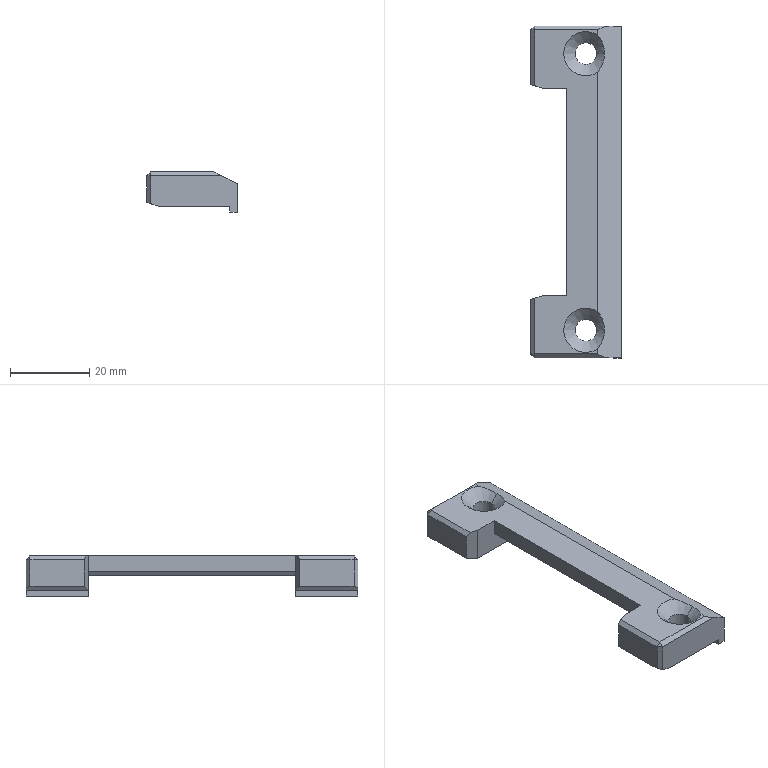Part | NX | features BREP 1 | 1 solid | 38 faces | box 23 x 84 x 10.2 mm | volume 8537 mm3 | plane 30 | cone 4 | cylinder 4 | commonest cylinder face diameters 5.5 x4
STEP:
#1=CARTESIAN_POINT('',(108.084,-207.077,2.15));
#2=VERTEX_POINT('',#1);
#3=CARTESIAN_POINT('',(113.584,-207.077,2.15));
#4=VERTEX_POINT('',#3);
#5=CARTESIAN_POINT('',(110.834,-207.077,2.15));
#6=DIRECTION('',(0.,0.,1.));
#7=DIRECTION('',(1.,0.,0.));
#8=AXIS2_PLACEMENT_3D('',#5,#6,#7);
#9=CIRCLE('',#8,2.75);
#10=EDGE_CURVE('',#2,#4,#9,.T.);
#11=ORIENTED_EDGE('',*,*,#10,.F.);
#12=CARTESIAN_POINT('',(105.234,-207.077,5.));
#13=VERTEX_POINT('',#12);
#14=CARTESIAN_POINT('',(105.234,-207.077,5.));
#15=DIRECTION('',(-0.7071,0.,0.7071));
#16=VECTOR('',#15,1000.);
#17=LINE('',#14,#16);
#18=EDGE_CURVE('',#13,#2,#17,.F.);
#19=ORIENTED_EDGE('',*,*,#18,.F.);
#20=CARTESIAN_POINT('',(113.834,-211.806,5.));
#21=VERTEX_POINT('',#20);
#22=CARTESIAN_POINT('',(110.834,-207.077,5.));
#23=DIRECTION('',(0.,0.,1.));
#24=DIRECTION('',(1.,0.,0.));
#25=AXIS2_PLACEMENT_3D('',#22,#23,#24);
#26=CIRCLE('',#25,5.6);
#27=EDGE_CURVE('',#13,#21,#26,.T.);
#28=ORIENTED_EDGE('',*,*,#27,.T.);
#29=CARTESIAN_POINT('',(115.568,-207.077,4.133));
#30=VERTEX_POINT('',#29);
#31=CARTESIAN_POINT('',(113.834,-211.806,5.));
#32=CARTESIAN_POINT('',(114.971,-210.411,4.432));
#33=CARTESIAN_POINT('',(115.568,-208.784,4.133));
#34=CARTESIAN_POINT('',(115.568,-207.077,4.133));
#35=(BOUNDED_CURVE()B_SPLINE_CURVE(3,(#31,#32,#33,#34),.UNSPECIFIED.,.F.,.F.)B_SPLINE_CURVE_WITH_KNOTS((4,4),(2.527,3.142),.UNSPECIFIED.)CURVE()GEOMETRIC_REPRESENTATION_ITEM()RATIONAL_B_SPLINE_CURVE((1.,0.9688,0.9688,1.))REPRESENTATION_ITEM(''));
#36=EDGE_CURVE('',#21,#30,#35,.T.);
#37=ORIENTED_EDGE('',*,*,#36,.T.);
#38=CARTESIAN_POINT('',(116.434,-207.077,5.));
#39=DIRECTION('',(0.7071,0.,0.7071));
#40=VECTOR('',#39,1000.);
#41=LINE('',#38,#40);
#42=EDGE_CURVE('',#30,#4,#41,.F.);
#43=ORIENTED_EDGE('',*,*,#42,.T.);
#44=EDGE_LOOP('',(#11,#19,#28,#37,#43));
#45=FACE_BOUND('',#44,.T.);
#46=CARTESIAN_POINT('',(110.834,-207.077,5.));
#47=DIRECTION('',(0.,0.,1.));
#48=DIRECTION('',(1.,0.,0.));
#49=AXIS2_PLACEMENT_3D('',#46,#47,#48);
#50=CONICAL_SURFACE('',#49,5.6,0.7854);
#51=ADVANCED_FACE('',(#45),#50,.F.);
#52=CARTESIAN_POINT('',(113.584,-207.077,-3.7));
#53=VERTEX_POINT('',#52);
#54=CARTESIAN_POINT('',(108.084,-207.077,-3.7));
#55=VERTEX_POINT('',#54);
#56=CARTESIAN_POINT('',(110.834,-207.077,-3.7));
#57=DIRECTION('',(0.,0.,-1.));
#58=DIRECTION('',(-1.,0.,0.));
#59=AXIS2_PLACEMENT_3D('',#56,#57,#58);
#60=CIRCLE('',#59,2.75);
#61=EDGE_CURVE('',#53,#55,#60,.T.);
#62=ORIENTED_EDGE('',*,*,#61,.T.);
#63=CARTESIAN_POINT('',(108.084,-207.077,5.));
#64=DIRECTION('',(0.,0.,1.));
#65=VECTOR('',#64,1000.);
#66=LINE('',#63,#65);
#67=EDGE_CURVE('',#2,#55,#66,.F.);
#68=ORIENTED_EDGE('',*,*,#67,.F.);
#69=ORIENTED_EDGE('',*,*,#10,.T.);
#70=CARTESIAN_POINT('',(113.584,-207.077,5.));
#71=DIRECTION('',(0.,0.,1.));
#72=VECTOR('',#71,1000.);
#73=LINE('',#70,#72);
#74=EDGE_CURVE('',#4,#53,#73,.F.);
#75=ORIENTED_EDGE('',*,*,#74,.T.);
#76=EDGE_LOOP('',(#62,#68,#69,#75));
#77=FACE_BOUND('',#76,.T.);
#78=CARTESIAN_POINT('',(110.834,-207.077,5.));
#79=DIRECTION('',(0.,0.,1.));
#80=DIRECTION('',(1.,0.,0.));
#81=AXIS2_PLACEMENT_3D('',#78,#79,#80);
#82=CYLINDRICAL_SURFACE('',#81,2.75);
#83=ADVANCED_FACE('',(#77),#82,.F.);
#84=CARTESIAN_POINT('',(108.084,-277.077,2.15));
#85=VERTEX_POINT('',#84);
#86=CARTESIAN_POINT('',(113.584,-277.077,2.15));
#87=VERTEX_POINT('',#86);
#88=CARTESIAN_POINT('',(110.834,-277.077,2.15));
#89=DIRECTION('',(0.,0.,1.));
#90=DIRECTION('',(1.,0.,0.));
#91=AXIS2_PLACEMENT_3D('',#88,#89,#90);
#92=CIRCLE('',#91,2.75);
#93=EDGE_CURVE('',#85,#87,#92,.T.);
#94=ORIENTED_EDGE('',*,*,#93,.F.);
#95=CARTESIAN_POINT('',(105.234,-277.077,5.));
#96=VERTEX_POINT('',#95);
#97=CARTESIAN_POINT('',(105.234,-277.077,5.));
#98=DIRECTION('',(-0.7071,0.,0.7071));
#99=VECTOR('',#98,1000.);
#100=LINE('',#97,#99);
#101=EDGE_CURVE('',#96,#85,#100,.F.);
#102=ORIENTED_EDGE('',*,*,#101,.F.);
#103=CARTESIAN_POINT('',(113.834,-281.806,5.));
#104=VERTEX_POINT('',#103);
#105=CARTESIAN_POINT('',(110.834,-277.077,5.));
#106=DIRECTION('',(0.,0.,1.));
#107=DIRECTION('',(1.,0.,0.));
#108=AXIS2_PLACEMENT_3D('',#105,#106,#107);
#109=CIRCLE('',#108,5.6);
#110=EDGE_CURVE('',#96,#104,#109,.T.);
#111=ORIENTED_EDGE('',*,*,#110,.T.);
#112=CARTESIAN_POINT('',(115.568,-277.077,4.133));
#113=VERTEX_POINT('',#112);
#114=CARTESIAN_POINT('',(113.834,-281.806,5.));
#115=CARTESIAN_POINT('',(114.971,-280.411,4.432));
#116=CARTESIAN_POINT('',(115.568,-278.784,4.133));
#117=CARTESIAN_POINT('',(115.568,-277.077,4.133));
#118=(BOUNDED_CURVE()B_SPLINE_CURVE(3,(#114,#115,#116,#117),.UNSPECIFIED.,.F.,.F.)B_SPLINE_CURVE_WITH_KNOTS((4,4),(2.527,3.142),.UNSPECIFIED.)CURVE()GEOMETRIC_REPRESENTATION_ITEM()RATIONAL_B_SPLINE_CURVE((1.,0.9688,0.9688,1.))REPRESENTATION_ITEM(''));
#119=EDGE_CURVE('',#104,#113,#118,.T.);
#120=ORIENTED_EDGE('',*,*,#119,.T.);
#121=CARTESIAN_POINT('',(116.434,-277.077,5.));
#122=DIRECTION('',(0.7071,0.,0.7071));
#123=VECTOR('',#122,1000.);
#124=LINE('',#121,#123);
#125=EDGE_CURVE('',#113,#87,#124,.F.);
#126=ORIENTED_EDGE('',*,*,#125,.T.);
#127=EDGE_LOOP('',(#94,#102,#111,#120,#126));
#128=FACE_BOUND('',#127,.T.);
#129=CARTESIAN_POINT('',(110.834,-277.077,5.));
#130=DIRECTION('',(0.,0.,1.));
#131=DIRECTION('',(1.,0.,0.));
#132=AXIS2_PLACEMENT_3D('',#129,#130,#131);
#133=CONICAL_SURFACE('',#132,5.6,0.7854);
#134=ADVANCED_FACE('',(#128),#133,.F.);
#135=CARTESIAN_POINT('',(108.084,-277.077,-3.7));
#136=VERTEX_POINT('',#135);
#137=CARTESIAN_POINT('',(113.584,-277.077,-3.7));
#138=VERTEX_POINT('',#137);
#139=CARTESIAN_POINT('',(110.834,-277.077,-3.7));
#140=DIRECTION('',(0.,0.,1.));
#141=DIRECTION('',(1.,0.,0.));
#142=AXIS2_PLACEMENT_3D('',#139,#140,#141);
#143=CIRCLE('',#142,2.75);
#144=EDGE_CURVE('',#136,#138,#143,.T.);
#145=ORIENTED_EDGE('',*,*,#144,.F.);
#146=CARTESIAN_POINT('',(108.084,-277.077,5.));
#147=DIRECTION('',(0.,0.,1.));
#148=VECTOR('',#147,1000.);
#149=LINE('',#146,#148);
#150=EDGE_CURVE('',#85,#136,#149,.F.);
#151=ORIENTED_EDGE('',*,*,#150,.F.);
#152=ORIENTED_EDGE('',*,*,#93,.T.);
#153=CARTESIAN_POINT('',(113.584,-277.077,5.));
#154=DIRECTION('',(0.,0.,1.));
#155=VECTOR('',#154,1000.);
#156=LINE('',#153,#155);
#157=EDGE_CURVE('',#87,#138,#156,.F.);
#158=ORIENTED_EDGE('',*,*,#157,.T.);
#159=EDGE_LOOP('',(#145,#151,#152,#158));
#160=FACE_BOUND('',#159,.T.);
#161=CARTESIAN_POINT('',(110.834,-277.077,5.));
#162=DIRECTION('',(0.,0.,1.));
#163=DIRECTION('',(1.,0.,0.));
#164=AXIS2_PLACEMENT_3D('',#161,#162,#163);
#165=CYLINDRICAL_SURFACE('',#164,2.75);
#166=ADVANCED_FACE('',(#160),#165,.F.);
#167=CARTESIAN_POINT('',(97.834,-268.994,5.));
#168=VERTEX_POINT('',#167);
#169=CARTESIAN_POINT('',(97.834,-283.077,5.));
#170=VERTEX_POINT('',#169);
#171=CARTESIAN_POINT('',(97.834,-284.077,5.));
#172=DIRECTION('',(0.,-1.,0.));
#173=VECTOR('',#172,1000.);
#174=LINE('',#171,#173);
#175=EDGE_CURVE('',#168,#170,#174,.T.);
#176=ORIENTED_EDGE('',*,*,#175,.T.);
#177=CARTESIAN_POINT('',(113.834,-283.077,5.));
#178=VERTEX_POINT('',#177);
#179=CARTESIAN_POINT('',(105.834,-283.077,5.));
#180=DIRECTION('',(1.,0.,0.));
#181=VECTOR('',#180,1000.);
#182=LINE('',#179,#181);
#183=EDGE_CURVE('',#170,#178,#182,.T.);
#184=ORIENTED_EDGE('',*,*,#183,.T.);
#185=CARTESIAN_POINT('',(113.834,-200.077,5.));
#186=DIRECTION('',(0.,1.,0.));
#187=VECTOR('',#186,1000.);
#188=LINE('',#185,#187);
#189=EDGE_CURVE('',#178,#104,#188,.T.);
#190=ORIENTED_EDGE('',*,*,#189,.T.);
#191=ORIENTED_EDGE('',*,*,#110,.F.);
#192=CARTESIAN_POINT('',(113.834,-272.349,5.));
#193=VERTEX_POINT('',#192);
#194=CARTESIAN_POINT('',(110.834,-277.077,5.));
#195=DIRECTION('',(0.,0.,1.));
#196=DIRECTION('',(1.,0.,0.));
#197=AXIS2_PLACEMENT_3D('',#194,#195,#196);
#198=CIRCLE('',#197,5.6);
#199=EDGE_CURVE('',#193,#96,#198,.T.);
#200=ORIENTED_EDGE('',*,*,#199,.F.);
#201=CARTESIAN_POINT('',(113.834,-200.077,5.));
#202=DIRECTION('',(0.,1.,0.));
#203=VECTOR('',#202,1000.);
#204=LINE('',#201,#203);
#205=EDGE_CURVE('',#193,#21,#204,.T.);
#206=ORIENTED_EDGE('',*,*,#205,.T.);
#207=ORIENTED_EDGE('',*,*,#27,.F.);
#208=CARTESIAN_POINT('',(113.834,-202.349,5.));
#209=VERTEX_POINT('',#208);
#210=CARTESIAN_POINT('',(110.834,-207.077,5.));
#211=DIRECTION('',(0.,0.,1.));
#212=DIRECTION('',(1.,0.,0.));
#213=AXIS2_PLACEMENT_3D('',#210,#211,#212);
#214=CIRCLE('',#213,5.6);
#215=EDGE_CURVE('',#209,#13,#214,.T.);
#216=ORIENTED_EDGE('',*,*,#215,.F.);
#217=CARTESIAN_POINT('',(113.834,-201.077,5.));
#218=VERTEX_POINT('',#217);
#219=CARTESIAN_POINT('',(113.834,-200.077,5.));
#220=DIRECTION('',(0.,1.,0.));
#221=VECTOR('',#220,1000.);
#222=LINE('',#219,#221);
#223=EDGE_CURVE('',#209,#218,#222,.T.);
#224=ORIENTED_EDGE('',*,*,#223,.T.);
#225=CARTESIAN_POINT('',(97.834,-201.077,5.));
#226=VERTEX_POINT('',#225);
#227=CARTESIAN_POINT('',(105.834,-201.077,5.));
#228=DIRECTION('',(-1.,0.,0.));
#229=VECTOR('',#228,1000.);
#230=LINE('',#227,#229);
#231=EDGE_CURVE('',#218,#226,#230,.T.);
#232=ORIENTED_EDGE('',*,*,#231,.T.);
#233=CARTESIAN_POINT('',(97.834,-215.161,5.));
#234=VERTEX_POINT('',#233);
#235=CARTESIAN_POINT('',(97.834,-200.077,5.));
#236=DIRECTION('',(0.,-1.,0.));
#237=VECTOR('',#236,1000.);
#238=LINE('',#235,#237);
#239=EDGE_CURVE('',#226,#234,#238,.T.);
#240=ORIENTED_EDGE('',*,*,#239,.T.);
#241=CARTESIAN_POINT('',(99.834,-215.827,5.));
#242=VERTEX_POINT('',#241);
#243=CARTESIAN_POINT('',(96.834,-214.827,5.));
#244=DIRECTION('',(0.9487,-0.3162,0.));
#245=VECTOR('',#244,1000.);
#246=LINE('',#243,#245);
#247=EDGE_CURVE('',#234,#242,#246,.T.);
#248=ORIENTED_EDGE('',*,*,#247,.T.);
#249=CARTESIAN_POINT('',(105.834,-215.827,5.));
#250=VERTEX_POINT('',#249);
#251=CARTESIAN_POINT('',(96.834,-215.827,5.));
#252=DIRECTION('',(1.,0.,0.));
#253=VECTOR('',#252,1000.);
#254=LINE('',#251,#253);
#255=EDGE_CURVE('',#242,#250,#254,.T.);
#256=ORIENTED_EDGE('',*,*,#255,.T.);
#257=CARTESIAN_POINT('',(105.834,-268.327,5.));
#258=VERTEX_POINT('',#257);
#259=CARTESIAN_POINT('',(105.834,-284.077,5.));
#260=DIRECTION('',(0.,-1.,0.));
#261=VECTOR('',#260,1000.);
#262=LINE('',#259,#261);
#263=EDGE_CURVE('',#250,#258,#262,.T.);
#264=ORIENTED_EDGE('',*,*,#263,.T.);
#265=CARTESIAN_POINT('',(99.834,-268.327,5.));
#266=VERTEX_POINT('',#265);
#267=CARTESIAN_POINT('',(96.834,-268.327,5.));
#268=DIRECTION('',(1.,0.,0.));
#269=VECTOR('',#268,1000.);
#270=LINE('',#267,#269);
#271=EDGE_CURVE('',#266,#258,#270,.T.);
#272=ORIENTED_EDGE('',*,*,#271,.F.);
#273=CARTESIAN_POINT('',(96.834,-269.327,5.));
#274=DIRECTION('',(-0.9487,-0.3162,0.));
#275=VECTOR('',#274,1000.);
#276=LINE('',#273,#275);
#277=EDGE_CURVE('',#266,#168,#276,.T.);
#278=ORIENTED_EDGE('',*,*,#277,.T.);
#279=EDGE_LOOP('',(#176,#184,#190,#191,#200,#206,#207,#216,#224,#232,#240,#248,#256,#264,#272,#278));
#280=FACE_BOUND('',#279,.T.);
#281=CARTESIAN_POINT('',(105.834,-200.077,5.));
#282=DIRECTION('',(0.,0.,-1.));
#283=DIRECTION('',(0.,-1.,0.));
#284=AXIS2_PLACEMENT_3D('',#281,#282,#283);
#285=PLANE('',#284);
#286=ADVANCED_FACE('',(#280),#285,.F.);
#287=CARTESIAN_POINT('',(117.834,-284.077,-3.7));
#288=VERTEX_POINT('',#287);
#289=CARTESIAN_POINT('',(117.834,-268.327,-3.7));
#290=VERTEX_POINT('',#289);
#291=CARTESIAN_POINT('',(117.834,-284.077,-3.7));
#292=DIRECTION('',(0.,1.,0.));
#293=VECTOR('',#292,1000.);
#294=LINE('',#291,#293);
#295=EDGE_CURVE('',#288,#290,#294,.T.);
#296=ORIENTED_EDGE('',*,*,#295,.F.);
#297=CARTESIAN_POINT('',(99.834,-284.077,-3.7));
#298=VERTEX_POINT('',#297);
#299=CARTESIAN_POINT('',(119.834,-284.077,-3.7));
#300=DIRECTION('',(-1.,0.,0.));
#301=VECTOR('',#300,1000.);
#302=LINE('',#299,#301);
#303=EDGE_CURVE('',#288,#298,#302,.T.);
#304=ORIENTED_EDGE('',*,*,#303,.T.);
#305=CARTESIAN_POINT('',(99.834,-268.327,-3.7));
#306=VERTEX_POINT('',#305);
#307=CARTESIAN_POINT('',(99.834,-268.327,-3.7));
#308=DIRECTION('',(0.,1.,0.));
#309=VECTOR('',#308,1000.);
#310=LINE('',#307,#309);
#311=EDGE_CURVE('',#298,#306,#310,.T.);
#312=ORIENTED_EDGE('',*,*,#311,.T.);
#313=CARTESIAN_POINT('',(119.834,-268.327,-3.7));
#314=DIRECTION('',(1.,0.,0.));
#315=VECTOR('',#314,1000.);
#316=LINE('',#313,#315);
#317=EDGE_CURVE('',#306,#290,#316,.T.);
#318=ORIENTED_EDGE('',*,*,#317,.T.);
#319=EDGE_LOOP('',(#296,#304,#312,#318));
#320=FACE_BOUND('',#319,.T.);
#321=CARTESIAN_POINT('',(110.834,-277.077,-3.7));
#322=DIRECTION('',(0.,0.,1.));
#323=DIRECTION('',(1.,0.,0.));
#324=AXIS2_PLACEMENT_3D('',#321,#322,#323);
#325=CIRCLE('',#324,2.75);
#326=EDGE_CURVE('',#138,#136,#325,.T.);
#327=ORIENTED_EDGE('',*,*,#326,.T.);
#328=ORIENTED_EDGE('',*,*,#144,.T.);
#329=EDGE_LOOP('',(#327,#328));
#330=FACE_BOUND('',#329,.T.);
#331=CARTESIAN_POINT('',(119.834,-268.327,-3.7));
#332=DIRECTION('',(0.,0.,1.));
#333=DIRECTION('',(1.,0.,0.));
#334=AXIS2_PLACEMENT_3D('',#331,#332,#333);
#335=PLANE('',#334);
#336=ADVANCED_FACE('',(#320,#330),#335,.F.);
#337=CARTESIAN_POINT('',(99.834,-200.077,-3.7));
#338=VERTEX_POINT('',#337);
#339=CARTESIAN_POINT('',(117.834,-200.077,-3.7));
#340=VERTEX_POINT('',#339);
#341=CARTESIAN_POINT('',(119.834,-200.077,-3.7));
#342=DIRECTION('',(1.,0.,0.));
#343=VECTOR('',#342,1000.);
#344=LINE('',#341,#343);
#345=EDGE_CURVE('',#338,#340,#344,.T.);
#346=ORIENTED_EDGE('',*,*,#345,.T.);
#347=CARTESIAN_POINT('',(117.834,-215.827,-3.7));
#348=VERTEX_POINT('',#347);
#349=CARTESIAN_POINT('',(117.834,-200.077,-3.7));
#350=DIRECTION('',(0.,1.,0.));
#351=VECTOR('',#350,1000.);
#352=LINE('',#349,#351);
#353=EDGE_CURVE('',#348,#340,#352,.T.);
#354=ORIENTED_EDGE('',*,*,#353,.F.);
#355=CARTESIAN_POINT('',(99.834,-215.827,-3.7));
#356=VERTEX_POINT('',#355);
#357=CARTESIAN_POINT('',(119.834,-215.827,-3.7));
#358=DIRECTION('',(-1.,0.,0.));
#359=VECTOR('',#358,1000.);
#360=LINE('',#357,#359);
#361=EDGE_CURVE('',#348,#356,#360,.T.);
#362=ORIENTED_EDGE('',*,*,#361,.T.);
#363=CARTESIAN_POINT('',(99.834,-200.077,-3.7));
#364=DIRECTION('',(0.,1.,0.));
#365=VECTOR('',#364,1000.);
#366=LINE('',#363,#365);
#367=EDGE_CURVE('',#356,#338,#366,.T.);
#368=ORIENTED_EDGE('',*,*,#367,.T.);
#369=EDGE_LOOP('',(#346,#354,#362,#368));
#370=FACE_BOUND('',#369,.T.);
#371=ORIENTED_EDGE('',*,*,#61,.F.);
#372=CARTESIAN_POINT('',(110.834,-207.077,-3.7));
#373=DIRECTION('',(0.,0.,-1.));
#374=DIRECTION('',(-1.,0.,0.));
#375=AXIS2_PLACEMENT_3D('',#372,#373,#374);
#376=CIRCLE('',#375,2.75);
#377=EDGE_CURVE('',#55,#53,#376,.T.);
#378=ORIENTED_EDGE('',*,*,#377,.F.);
#379=EDGE_LOOP('',(#371,#378));
#380=FACE_BOUND('',#379,.T.);
#381=CARTESIAN_POINT('',(119.834,-215.827,-3.7));
#382=DIRECTION('',(0.,0.,-1.));
#383=DIRECTION('',(0.,-1.,0.));
#384=AXIS2_PLACEMENT_3D('',#381,#382,#383);
#385=PLANE('',#384);
#386=ADVANCED_FACE('',(#370,#380),#385,.T.);
#387=CARTESIAN_POINT('',(105.834,-215.827,1.));
#388=VERTEX_POINT('',#387);
#389=CARTESIAN_POINT('',(105.834,-215.827,-3.7));
#390=DIRECTION('',(0.,0.,1.));
#391=VECTOR('',#390,1000.);
#392=LINE('',#389,#391);
#393=EDGE_CURVE('',#388,#250,#392,.T.);
#394=ORIENTED_EDGE('',*,*,#393,.F.);
#395=CARTESIAN_POINT('',(105.834,-268.327,1.));
#396=VERTEX_POINT('',#395);
#397=CARTESIAN_POINT('',(105.834,-268.327,1.));
#398=DIRECTION('',(0.,-1.,0.));
#399=VECTOR('',#398,1000.);
#400=LINE('',#397,#399);
#401=EDGE_CURVE('',#388,#396,#400,.T.);
#402=ORIENTED_EDGE('',*,*,#401,.T.);
#403=CARTESIAN_POINT('',(105.834,-268.327,-3.7));
#404=DIRECTION('',(0.,0.,-1.));
#405=VECTOR('',#404,1000.);
#406=LINE('',#403,#405);
#407=EDGE_CURVE('',#258,#396,#406,.T.);
#408=ORIENTED_EDGE('',*,*,#407,.F.);
#409=ORIENTED_EDGE('',*,*,#263,.F.);
#410=EDGE_LOOP('',(#394,#402,#408,#409));
#411=FACE_BOUND('',#410,.T.);
#412=CARTESIAN_POINT('',(105.834,-284.077,5.));
#413=DIRECTION('',(1.,0.,0.));
#414=DIRECTION('',(0.,1.,0.));
#415=AXIS2_PLACEMENT_3D('',#412,#413,#414);
#416=PLANE('',#415);
#417=ADVANCED_FACE('',(#411),#416,.F.);
#418=CARTESIAN_POINT('',(108.834,-268.327,0.));
#419=VERTEX_POINT('',#418);
#420=CARTESIAN_POINT('',(119.834,-268.327,0.));
#421=VERTEX_POINT('',#420);
#422=CARTESIAN_POINT('',(119.834,-268.327,0.));
#423=DIRECTION('',(1.,0.,0.));
#424=VECTOR('',#423,1000.);
#425=LINE('',#422,#424);
#426=EDGE_CURVE('',#419,#421,#425,.T.);
#427=ORIENTED_EDGE('',*,*,#426,.F.);
#428=CARTESIAN_POINT('',(108.834,-215.827,0.));
#429=VERTEX_POINT('',#428);
#430=CARTESIAN_POINT('',(108.834,-215.827,0.));
#431=DIRECTION('',(0.,1.,0.));
#432=VECTOR('',#431,1000.);
#433=LINE('',#430,#432);
#434=EDGE_CURVE('',#419,#429,#433,.T.);
#435=ORIENTED_EDGE('',*,*,#434,.T.);
#436=CARTESIAN_POINT('',(119.834,-215.827,0.));
#437=VERTEX_POINT('',#436);
#438=CARTESIAN_POINT('',(119.834,-215.827,0.));
#439=DIRECTION('',(-1.,0.,0.));
#440=VECTOR('',#439,1000.);
#441=LINE('',#438,#440);
#442=EDGE_CURVE('',#437,#429,#441,.T.);
#443=ORIENTED_EDGE('',*,*,#442,.F.);
#444=CARTESIAN_POINT('',(119.834,-284.077,0.));
#445=DIRECTION('',(0.,1.,0.));
#446=VECTOR('',#445,1000.);
#447=LINE('',#444,#446);
#448=EDGE_CURVE('',#421,#437,#447,.T.);
#449=ORIENTED_EDGE('',*,*,#448,.F.);
#450=EDGE_LOOP('',(#427,#435,#443,#449));
#451=FACE_BOUND('',#450,.T.);
#452=CARTESIAN_POINT('',(105.834,-200.077,0.));
#453=DIRECTION('',(0.,0.,-1.));
#454=DIRECTION('',(0.,-1.,0.));
#455=AXIS2_PLACEMENT_3D('',#452,#453,#454);
#456=PLANE('',#455);
#457=ADVANCED_FACE('',(#451),#456,.T.);
#458=CARTESIAN_POINT('',(119.834,-284.077,2.));
#459=VERTEX_POINT('',#458);
#460=CARTESIAN_POINT('',(115.834,-284.077,4.));
#461=VERTEX_POINT('',#460);
#462=CARTESIAN_POINT('',(113.834,-284.077,5.));
#463=DIRECTION('',(-0.8944,0.,0.4472));
#464=VECTOR('',#463,1000.);
#465=LINE('',#462,#464);
#466=EDGE_CURVE('',#459,#461,#465,.T.);
#467=ORIENTED_EDGE('',*,*,#466,.T.);
#468=CARTESIAN_POINT('',(97.834,-284.077,4.));
#469=VERTEX_POINT('',#468);
#470=CARTESIAN_POINT('',(105.834,-284.077,4.));
#471=DIRECTION('',(-1.,0.,0.));
#472=VECTOR('',#471,1000.);
#473=LINE('',#470,#472);
#474=EDGE_CURVE('',#461,#469,#473,.T.);
#475=ORIENTED_EDGE('',*,*,#474,.T.);
#476=CARTESIAN_POINT('',(97.834,-284.077,-3.033));
#477=VERTEX_POINT('',#476);
#478=CARTESIAN_POINT('',(97.834,-284.077,-2.7));
#479=DIRECTION('',(0.,0.,-1.));
#480=VECTOR('',#479,1000.);
#481=LINE('',#478,#480);
#482=EDGE_CURVE('',#469,#477,#481,.T.);
#483=ORIENTED_EDGE('',*,*,#482,.T.);
#484=CARTESIAN_POINT('',(96.834,-284.077,-2.7));
#485=DIRECTION('',(0.9487,0.,-0.3162));
#486=VECTOR('',#485,1000.);
#487=LINE('',#484,#486);
#488=EDGE_CURVE('',#477,#298,#487,.T.);
#489=ORIENTED_EDGE('',*,*,#488,.T.);
#490=ORIENTED_EDGE('',*,*,#303,.F.);
#491=CARTESIAN_POINT('',(117.834,-284.077,-5.2));
#492=VERTEX_POINT('',#491);
#493=CARTESIAN_POINT('',(117.834,-284.077,-5.2));
#494=DIRECTION('',(0.,0.,1.));
#495=VECTOR('',#494,1000.);
#496=LINE('',#493,#495);
#497=EDGE_CURVE('',#492,#288,#496,.T.);
#498=ORIENTED_EDGE('',*,*,#497,.F.);
#499=CARTESIAN_POINT('',(119.834,-284.077,-5.2));
#500=VERTEX_POINT('',#499);
#501=CARTESIAN_POINT('',(119.834,-284.077,-5.2));
#502=DIRECTION('',(-1.,0.,0.));
#503=VECTOR('',#502,1000.);
#504=LINE('',#501,#503);
#505=EDGE_CURVE('',#500,#492,#504,.T.);
#506=ORIENTED_EDGE('',*,*,#505,.F.);
#507=CARTESIAN_POINT('',(119.834,-284.077,5.));
#508=DIRECTION('',(0.,0.,-1.));
#509=VECTOR('',#508,1000.);
#510=LINE('',#507,#509);
#511=EDGE_CURVE('',#459,#500,#510,.T.);
#512=ORIENTED_EDGE('',*,*,#511,.F.);
#513=EDGE_LOOP('',(#467,#475,#483,#489,#490,#498,#506,#512));
#514=FACE_BOUND('',#513,.T.);
#515=CARTESIAN_POINT('',(105.834,-284.077,5.));
#516=DIRECTION('',(0.,1.,0.));
#517=DIRECTION('',(1.,0.,0.));
#518=AXIS2_PLACEMENT_3D('',#515,#516,#517);
#519=PLANE('',#518);
#520=ADVANCED_FACE('',(#514),#519,.F.);
#521=CARTESIAN_POINT('',(119.834,-200.077,2.));
#522=VERTEX_POINT('',#521);
#523=CARTESIAN_POINT('',(119.834,-200.077,-5.2));
#524=VERTEX_POINT('',#523);
#525=CARTESIAN_POINT('',(119.834,-200.077,5.));
#526=DIRECTION('',(0.,0.,-1.));
#527=VECTOR('',#526,1000.);
#528=LINE('',#525,#527);
#529=EDGE_CURVE('',#522,#524,#528,.T.);
#530=ORIENTED_EDGE('',*,*,#529,.F.);
#531=CARTESIAN_POINT('',(119.834,-284.077,2.));
#532=DIRECTION('',(0.,-1.,0.));
#533=VECTOR('',#532,1000.);
#534=LINE('',#531,#533);
#535=EDGE_CURVE('',#522,#459,#534,.T.);
#536=ORIENTED_EDGE('',*,*,#535,.T.);
#537=ORIENTED_EDGE('',*,*,#511,.T.);
#538=CARTESIAN_POINT('',(119.834,-268.327,-5.2));
#539=VERTEX_POINT('',#538);
#540=CARTESIAN_POINT('',(119.834,-284.077,-5.2));
#541=DIRECTION('',(0.,-1.,0.));
#542=VECTOR('',#541,1000.);
#543=LINE('',#540,#542);
#544=EDGE_CURVE('',#539,#500,#543,.T.);
#545=ORIENTED_EDGE('',*,*,#544,.F.);
#546=CARTESIAN_POINT('',(119.834,-268.327,-3.7));
#547=DIRECTION('',(0.,0.,1.));
#548=VECTOR('',#547,1000.);
#549=LINE('',#546,#548);
#550=EDGE_CURVE('',#539,#421,#549,.T.);
#551=ORIENTED_EDGE('',*,*,#550,.T.);
#552=ORIENTED_EDGE('',*,*,#448,.T.);
#553=CARTESIAN_POINT('',(119.834,-215.827,-5.2));
#554=VERTEX_POINT('',#553);
#555=CARTESIAN_POINT('',(119.834,-215.827,-3.7));
#556=DIRECTION('',(0.,0.,1.));
#557=VECTOR('',#556,1000.);
#558=LINE('',#555,#557);
#559=EDGE_CURVE('',#554,#437,#558,.T.);
#560=ORIENTED_EDGE('',*,*,#559,.F.);
#561=CARTESIAN_POINT('',(119.834,-200.077,-5.2));
#562=DIRECTION('',(0.,-1.,0.));
#563=VECTOR('',#562,1000.);
#564=LINE('',#561,#563);
#565=EDGE_CURVE('',#524,#554,#564,.T.);
#566=ORIENTED_EDGE('',*,*,#565,.F.);
#567=EDGE_LOOP('',(#530,#536,#537,#545,#551,#552,#560,#566));
#568=FACE_BOUND('',#567,.T.);
#569=CARTESIAN_POINT('',(119.834,-284.077,5.));
#570=DIRECTION('',(-1.,0.,0.));
#571=DIRECTION('',(0.,0.,1.));
#572=AXIS2_PLACEMENT_3D('',#569,#570,#571);
#573=PLANE('',#572);
#574=ADVANCED_FACE('',(#568),#573,.F.);
#575=CARTESIAN_POINT('',(97.834,-200.077,-3.033));
#576=VERTEX_POINT('',#575);
#577=CARTESIAN_POINT('',(97.834,-200.077,4.));
#578=VERTEX_POINT('',#577);
#579=CARTESIAN_POINT('',(97.834,-200.077,5.));
#580=DIRECTION('',(0.,0.,1.));
#581=VECTOR('',#580,1000.);
#582=LINE('',#579,#581);
#583=EDGE_CURVE('',#576,#578,#582,.T.);
#584=ORIENTED_EDGE('',*,*,#583,.T.);
#585=CARTESIAN_POINT('',(115.834,-200.077,4.));
#586=VERTEX_POINT('',#585);
#587=CARTESIAN_POINT('',(105.834,-200.077,4.));
#588=DIRECTION('',(1.,0.,0.));
#589=VECTOR('',#588,1000.);
#590=LINE('',#587,#589);
#591=EDGE_CURVE('',#578,#586,#590,.T.);
#592=ORIENTED_EDGE('',*,*,#591,.T.);
#593=CARTESIAN_POINT('',(113.834,-200.077,5.));
#594=DIRECTION('',(0.8944,0.,-0.4472));
#595=VECTOR('',#594,1000.);
#596=LINE('',#593,#595);
#597=EDGE_CURVE('',#586,#522,#596,.T.);
#598=ORIENTED_EDGE('',*,*,#597,.T.);
#599=ORIENTED_EDGE('',*,*,#529,.T.);
#600=CARTESIAN_POINT('',(117.834,-200.077,-5.2));
#601=VERTEX_POINT('',#600);
#602=CARTESIAN_POINT('',(119.834,-200.077,-5.2));
#603=DIRECTION('',(1.,0.,0.));
#604=VECTOR('',#603,1000.);
#605=LINE('',#602,#604);
#606=EDGE_CURVE('',#601,#524,#605,.T.);
#607=ORIENTED_EDGE('',*,*,#606,.F.);
#608=CARTESIAN_POINT('',(117.834,-200.077,-5.2));
#609=DIRECTION('',(0.,0.,1.));
#610=VECTOR('',#609,1000.);
#611=LINE('',#608,#610);
#612=EDGE_CURVE('',#601,#340,#611,.T.);
#613=ORIENTED_EDGE('',*,*,#612,.T.);
#614=ORIENTED_EDGE('',*,*,#345,.F.);
#615=CARTESIAN_POINT('',(96.834,-200.077,-2.7));
#616=DIRECTION('',(-0.9487,0.,0.3162));
#617=VECTOR('',#616,1000.);
#618=LINE('',#615,#617);
#619=EDGE_CURVE('',#338,#576,#618,.T.);
#620=ORIENTED_EDGE('',*,*,#619,.T.);
#621=EDGE_LOOP('',(#584,#592,#598,#599,#607,#613,#614,#620));
#622=FACE_BOUND('',#621,.T.);
#623=CARTESIAN_POINT('',(105.834,-200.077,5.));
#624=DIRECTION('',(0.,-1.,0.));
#625=DIRECTION('',(0.,0.,-1.));
#626=AXIS2_PLACEMENT_3D('',#623,#624,#625);
#627=PLANE('',#626);
#628=ADVANCED_FACE('',(#622),#627,.F.);
#629=ORIENTED_EDGE('',*,*,#255,.F.);
#630=CARTESIAN_POINT('',(99.834,-215.827,-3.7));
#631=DIRECTION('',(0.,0.,-1.));
#632=VECTOR('',#631,1000.);
#633=LINE('',#630,#632);
#634=EDGE_CURVE('',#242,#356,#633,.T.);
#635=ORIENTED_EDGE('',*,*,#634,.T.);
#636=ORIENTED_EDGE('',*,*,#361,.F.);
#637=CARTESIAN_POINT('',(117.834,-215.827,-5.2));
#638=VERTEX_POINT('',#637);
#639=CARTESIAN_POINT('',(117.834,-215.827,-5.2));
#640=DIRECTION('',(0.,0.,1.));
#641=VECTOR('',#640,1000.);
#642=LINE('',#639,#641);
#643=EDGE_CURVE('',#638,#348,#642,.T.);
#644=ORIENTED_EDGE('',*,*,#643,.F.);
#645=CARTESIAN_POINT('',(119.834,-215.827,-5.2));
#646=DIRECTION('',(-1.,0.,0.));
#647=VECTOR('',#646,1000.);
#648=LINE('',#645,#647);
#649=EDGE_CURVE('',#554,#638,#648,.T.);
#650=ORIENTED_EDGE('',*,*,#649,.F.);
#651=ORIENTED_EDGE('',*,*,#559,.T.);
#652=ORIENTED_EDGE('',*,*,#442,.T.);
#653=CARTESIAN_POINT('',(119.844,-215.827,-3.67));
#654=DIRECTION('',(-0.9487,0.,0.3162));
#655=VECTOR('',#654,1000.);
#656=LINE('',#653,#655);
#657=EDGE_CURVE('',#429,#388,#656,.T.);
#658=ORIENTED_EDGE('',*,*,#657,.T.);
#659=ORIENTED_EDGE('',*,*,#393,.T.);
#660=EDGE_LOOP('',(#629,#635,#636,#644,#650,#651,#652,#658,#659));
#661=FACE_BOUND('',#660,.T.);
#662=CARTESIAN_POINT('',(119.834,-215.827,-3.7));
#663=DIRECTION('',(0.,1.,0.));
#664=DIRECTION('',(1.,0.,0.));
#665=AXIS2_PLACEMENT_3D('',#662,#663,#664);
#666=PLANE('',#665);
#667=ADVANCED_FACE('',(#661),#666,.F.);
#668=ORIENTED_EDGE('',*,*,#317,.F.);
#669=CARTESIAN_POINT('',(99.834,-268.327,5.));
#670=DIRECTION('',(0.,0.,1.));
#671=VECTOR('',#670,1000.);
#672=LINE('',#669,#671);
#673=EDGE_CURVE('',#306,#266,#672,.T.);
#674=ORIENTED_EDGE('',*,*,#673,.T.);
#675=ORIENTED_EDGE('',*,*,#271,.T.);
#676=ORIENTED_EDGE('',*,*,#407,.T.);
#677=CARTESIAN_POINT('',(119.844,-268.327,-3.67));
#678=DIRECTION('',(0.9487,0.,-0.3162));
#679=VECTOR('',#678,1000.);
#680=LINE('',#677,#679);
#681=EDGE_CURVE('',#396,#419,#680,.T.);
#682=ORIENTED_EDGE('',*,*,#681,.T.);
#683=ORIENTED_EDGE('',*,*,#426,.T.);
#684=ORIENTED_EDGE('',*,*,#550,.F.);
#685=CARTESIAN_POINT('',(117.834,-268.327,-5.2));
#686=VERTEX_POINT('',#685);
#687=CARTESIAN_POINT('',(119.834,-268.327,-5.2));
#688=DIRECTION('',(1.,0.,0.));
#689=VECTOR('',#688,1000.);
#690=LINE('',#687,#689);
#691=EDGE_CURVE('',#686,#539,#690,.T.);
#692=ORIENTED_EDGE('',*,*,#691,.F.);
#693=CARTESIAN_POINT('',(117.834,-268.327,-5.2));
#694=DIRECTION('',(0.,0.,1.));
#695=VECTOR('',#694,1000.);
#696=LINE('',#693,#695);
#697=EDGE_CURVE('',#686,#290,#696,.T.);
#698=ORIENTED_EDGE('',*,*,#697,.T.);
#699=EDGE_LOOP('',(#668,#674,#675,#676,#682,#683,#684,#692,#698));
#700=FACE_BOUND('',#699,.T.);
#701=CARTESIAN_POINT('',(119.834,-268.327,-3.7));
#702=DIRECTION('',(0.,-1.,0.));
#703=DIRECTION('',(0.,0.,-1.));
#704=AXIS2_PLACEMENT_3D('',#701,#702,#703);
#705=PLANE('',#704);
#706=ADVANCED_FACE('',(#700),#705,.F.);
#707=ORIENTED_EDGE('',*,*,#189,.F.);
#708=CARTESIAN_POINT('',(86.168,-269.244,18.833));
#709=DIRECTION('',(0.8165,-0.4082,-0.4082));
#710=VECTOR('',#709,1000.);
#711=LINE('',#708,#710);
#712=EDGE_CURVE('',#178,#461,#711,.T.);
#713=ORIENTED_EDGE('',*,*,#712,.T.);
#714=ORIENTED_EDGE('',*,*,#466,.F.);
#715=ORIENTED_EDGE('',*,*,#535,.F.);
#716=ORIENTED_EDGE('',*,*,#597,.F.);
#717=CARTESIAN_POINT('',(114.168,-200.911,4.833));
#718=DIRECTION('',(-0.8165,-0.4082,0.4082));
#719=VECTOR('',#718,1000.);
#720=LINE('',#717,#719);
#721=EDGE_CURVE('',#586,#218,#720,.T.);
#722=ORIENTED_EDGE('',*,*,#721,.T.);
#723=ORIENTED_EDGE('',*,*,#223,.F.);
#724=CARTESIAN_POINT('',(115.568,-207.077,4.133));
#725=CARTESIAN_POINT('',(115.568,-205.37,4.133));
#726=CARTESIAN_POINT('',(114.971,-203.743,4.432));
#727=CARTESIAN_POINT('',(113.834,-202.349,5.));
#728=(BOUNDED_CURVE()B_SPLINE_CURVE(3,(#724,#725,#726,#727),.UNSPECIFIED.,.F.,.F.)B_SPLINE_CURVE_WITH_KNOTS((4,4),(3.142,3.756),.UNSPECIFIED.)CURVE()GEOMETRIC_REPRESENTATION_ITEM()RATIONAL_B_SPLINE_CURVE((1.,0.9688,0.9688,1.))REPRESENTATION_ITEM(''));
#729=EDGE_CURVE('',#30,#209,#728,.T.);
#730=ORIENTED_EDGE('',*,*,#729,.F.);
#731=ORIENTED_EDGE('',*,*,#36,.F.);
#732=ORIENTED_EDGE('',*,*,#205,.F.);
#733=CARTESIAN_POINT('',(115.568,-277.077,4.133));
#734=CARTESIAN_POINT('',(115.568,-275.37,4.133));
#735=CARTESIAN_POINT('',(114.971,-273.743,4.432));
#736=CARTESIAN_POINT('',(113.834,-272.349,5.));
#737=(BOUNDED_CURVE()B_SPLINE_CURVE(3,(#733,#734,#735,#736),.UNSPECIFIED.,.F.,.F.)B_SPLINE_CURVE_WITH_KNOTS((4,4),(3.142,3.756),.UNSPECIFIED.)CURVE()GEOMETRIC_REPRESENTATION_ITEM()RATIONAL_B_SPLINE_CURVE((1.,0.9688,0.9688,1.))REPRESENTATION_ITEM(''));
#738=EDGE_CURVE('',#113,#193,#737,.T.);
#739=ORIENTED_EDGE('',*,*,#738,.F.);
#740=ORIENTED_EDGE('',*,*,#119,.F.);
#741=EDGE_LOOP('',(#707,#713,#714,#715,#716,#722,#723,#730,#731,#732,#739,#740));
#742=FACE_BOUND('',#741,.T.);
#743=CARTESIAN_POINT('',(113.834,-200.077,5.));
#744=DIRECTION('',(-0.4472,0.,-0.8944));
#745=DIRECTION('',(-0.8944,0.,0.4472));
#746=AXIS2_PLACEMENT_3D('',#743,#744,#745);
#747=PLANE('',#746);
#748=ADVANCED_FACE('',(#742),#747,.F.);
#749=CARTESIAN_POINT('',(96.834,-214.827,-2.7));
#750=VERTEX_POINT('',#749);
#751=CARTESIAN_POINT('',(96.834,-214.827,4.));
#752=VERTEX_POINT('',#751);
#753=CARTESIAN_POINT('',(96.834,-214.827,-3.7));
#754=DIRECTION('',(0.,0.,1.));
#755=VECTOR('',#754,1000.);
#756=LINE('',#753,#755);
#757=EDGE_CURVE('',#750,#752,#756,.T.);
#758=ORIENTED_EDGE('',*,*,#757,.T.);
#759=CARTESIAN_POINT('',(96.834,-201.077,4.));
#760=VERTEX_POINT('',#759);
#761=CARTESIAN_POINT('',(96.834,-200.077,4.));
#762=DIRECTION('',(0.,1.,0.));
#763=VECTOR('',#762,1000.);
#764=LINE('',#761,#763);
#765=EDGE_CURVE('',#752,#760,#764,.T.);
#766=ORIENTED_EDGE('',*,*,#765,.T.);
#767=CARTESIAN_POINT('',(96.834,-201.077,-2.7));
#768=VERTEX_POINT('',#767);
#769=CARTESIAN_POINT('',(96.834,-201.077,-3.7));
#770=DIRECTION('',(0.,0.,-1.));
#771=VECTOR('',#770,1000.);
#772=LINE('',#769,#771);
#773=EDGE_CURVE('',#760,#768,#772,.T.);
#774=ORIENTED_EDGE('',*,*,#773,.T.);
#775=CARTESIAN_POINT('',(96.834,-215.827,-2.7));
#776=DIRECTION('',(0.,-1.,0.));
#777=VECTOR('',#776,1000.);
#778=LINE('',#775,#777);
#779=EDGE_CURVE('',#768,#750,#778,.T.);
#780=ORIENTED_EDGE('',*,*,#779,.T.);
#781=EDGE_LOOP('',(#758,#766,#774,#780));
#782=FACE_BOUND('',#781,.T.);
#783=CARTESIAN_POINT('',(96.834,-200.077,-3.7));
#784=DIRECTION('',(1.,0.,0.));
#785=DIRECTION('',(0.,1.,0.));
#786=AXIS2_PLACEMENT_3D('',#783,#784,#785);
#787=PLANE('',#786);
#788=ADVANCED_FACE('',(#782),#787,.F.);
#789=CARTESIAN_POINT('',(96.834,-269.327,-2.7));
#790=VERTEX_POINT('',#789);
#791=CARTESIAN_POINT('',(96.834,-283.077,-2.7));
#792=VERTEX_POINT('',#791);
#793=CARTESIAN_POINT('',(96.834,-284.077,-2.7));
#794=DIRECTION('',(0.,-1.,0.));
#795=VECTOR('',#794,1000.);
#796=LINE('',#793,#795);
#797=EDGE_CURVE('',#790,#792,#796,.T.);
#798=ORIENTED_EDGE('',*,*,#797,.T.);
#799=CARTESIAN_POINT('',(96.834,-283.077,4.));
#800=VERTEX_POINT('',#799);
#801=CARTESIAN_POINT('',(96.834,-283.077,5.));
#802=DIRECTION('',(0.,0.,1.));
#803=VECTOR('',#802,1000.);
#804=LINE('',#801,#803);
#805=EDGE_CURVE('',#792,#800,#804,.T.);
#806=ORIENTED_EDGE('',*,*,#805,.T.);
#807=CARTESIAN_POINT('',(96.834,-269.327,4.));
#808=VERTEX_POINT('',#807);
#809=CARTESIAN_POINT('',(96.834,-269.327,4.));
#810=DIRECTION('',(0.,1.,0.));
#811=VECTOR('',#810,1000.);
#812=LINE('',#809,#811);
#813=EDGE_CURVE('',#800,#808,#812,.T.);
#814=ORIENTED_EDGE('',*,*,#813,.T.);
#815=CARTESIAN_POINT('',(96.834,-269.327,-3.7));
#816=DIRECTION('',(0.,0.,-1.));
#817=VECTOR('',#816,1000.);
#818=LINE('',#815,#817);
#819=EDGE_CURVE('',#808,#790,#818,.T.);
#820=ORIENTED_EDGE('',*,*,#819,.T.);
#821=EDGE_LOOP('',(#798,#806,#814,#820));
#822=FACE_BOUND('',#821,.T.);
#823=CARTESIAN_POINT('',(96.834,-284.077,-3.7));
#824=DIRECTION('',(-1.,0.,0.));
#825=DIRECTION('',(0.,0.,1.));
#826=AXIS2_PLACEMENT_3D('',#823,#824,#825);
#827=PLANE('',#826);
#828=ADVANCED_FACE('',(#822),#827,.T.);
#829=ORIENTED_EDGE('',*,*,#657,.F.);
#830=ORIENTED_EDGE('',*,*,#434,.F.);
#831=ORIENTED_EDGE('',*,*,#681,.F.);
#832=ORIENTED_EDGE('',*,*,#401,.F.);
#833=EDGE_LOOP('',(#829,#830,#831,#832));
#834=FACE_BOUND('',#833,.T.);
#835=CARTESIAN_POINT('',(105.834,-284.077,1.));
#836=DIRECTION('',(-0.3162,0.,-0.9487));
#837=DIRECTION('',(-0.9487,0.,0.3162));
#838=AXIS2_PLACEMENT_3D('',#835,#836,#837);
#839=PLANE('',#838);
#840=ADVANCED_FACE('',(#834),#839,.T.);
#841=ORIENTED_EDGE('',*,*,#247,.F.);
#842=CARTESIAN_POINT('',(93.187,-213.611,0.3526));
#843=DIRECTION('',(-0.6882,0.2294,-0.6882));
#844=VECTOR('',#843,1000.);
#845=LINE('',#842,#844);
#846=EDGE_CURVE('',#234,#752,#845,.T.);
#847=ORIENTED_EDGE('',*,*,#846,.T.);
#848=ORIENTED_EDGE('',*,*,#757,.F.);
#849=CARTESIAN_POINT('',(97.107,-214.918,-2.791));
#850=DIRECTION('',(-0.9045,0.3015,0.3015));
#851=VECTOR('',#850,1000.);
#852=LINE('',#849,#851);
#853=EDGE_CURVE('',#356,#750,#852,.T.);
#854=ORIENTED_EDGE('',*,*,#853,.F.);
#855=ORIENTED_EDGE('',*,*,#634,.F.);
#856=EDGE_LOOP('',(#841,#847,#848,#854,#855));
#857=FACE_BOUND('',#856,.T.);
#858=CARTESIAN_POINT('',(96.834,-214.827,-3.7));
#859=DIRECTION('',(0.3162,0.9487,0.));
#860=DIRECTION('',(0.,0.,-1.));
#861=AXIS2_PLACEMENT_3D('',#858,#859,#860);
#862=PLANE('',#861);
#863=ADVANCED_FACE('',(#857),#862,.F.);
#864=ORIENTED_EDGE('',*,*,#779,.F.);
#865=CARTESIAN_POINT('',(97.308,-200.604,-2.858));
#866=DIRECTION('',(0.6882,0.6882,-0.2294));
#867=VECTOR('',#866,1000.);
#868=LINE('',#865,#867);
#869=EDGE_CURVE('',#768,#576,#868,.T.);
#870=ORIENTED_EDGE('',*,*,#869,.T.);
#871=ORIENTED_EDGE('',*,*,#619,.F.);
#872=ORIENTED_EDGE('',*,*,#367,.F.);
#873=ORIENTED_EDGE('',*,*,#853,.T.);
#874=EDGE_LOOP('',(#864,#870,#871,#872,#873));
#875=FACE_BOUND('',#874,.T.);
#876=CARTESIAN_POINT('',(96.834,-200.077,-2.7));
#877=DIRECTION('',(-0.3162,0.,-0.9487));
#878=DIRECTION('',(-0.9487,0.,0.3162));
#879=AXIS2_PLACEMENT_3D('',#876,#877,#878);
#880=PLANE('',#879);
#881=ADVANCED_FACE('',(#875),#880,.T.);
#882=ORIENTED_EDGE('',*,*,#819,.F.);
#883=CARTESIAN_POINT('',(93.187,-270.543,0.3526));
#884=DIRECTION('',(0.6882,0.2294,0.6882));
#885=VECTOR('',#884,1000.);
#886=LINE('',#883,#885);
#887=EDGE_CURVE('',#808,#168,#886,.T.);
#888=ORIENTED_EDGE('',*,*,#887,.T.);
#889=ORIENTED_EDGE('',*,*,#277,.F.);
#890=ORIENTED_EDGE('',*,*,#673,.F.);
#891=CARTESIAN_POINT('',(97.107,-269.236,-2.791));
#892=DIRECTION('',(0.9045,0.3015,-0.3015));
#893=VECTOR('',#892,1000.);
#894=LINE('',#891,#893);
#895=EDGE_CURVE('',#790,#306,#894,.T.);
#896=ORIENTED_EDGE('',*,*,#895,.F.);
#897=EDGE_LOOP('',(#882,#888,#889,#890,#896));
#898=FACE_BOUND('',#897,.T.);
#899=CARTESIAN_POINT('',(96.834,-269.327,-3.7));
#900=DIRECTION('',(-0.3162,0.9487,0.));
#901=DIRECTION('',(0.,0.,1.));
#902=AXIS2_PLACEMENT_3D('',#899,#900,#901);
#903=PLANE('',#902);
#904=ADVANCED_FACE('',(#898),#903,.T.);
#905=ORIENTED_EDGE('',*,*,#488,.F.);
#906=CARTESIAN_POINT('',(97.308,-283.551,-2.858));
#907=DIRECTION('',(-0.6882,0.6882,0.2294));
#908=VECTOR('',#907,1000.);
#909=LINE('',#906,#908);
#910=EDGE_CURVE('',#477,#792,#909,.T.);
#911=ORIENTED_EDGE('',*,*,#910,.T.);
#912=ORIENTED_EDGE('',*,*,#797,.F.);
#913=ORIENTED_EDGE('',*,*,#895,.T.);
#914=ORIENTED_EDGE('',*,*,#311,.F.);
#915=EDGE_LOOP('',(#905,#911,#912,#913,#914));
#916=FACE_BOUND('',#915,.T.);
#917=CARTESIAN_POINT('',(96.834,-284.077,-2.7));
#918=DIRECTION('',(-0.3162,0.,-0.9487));
#919=DIRECTION('',(-0.9487,0.,0.3162));
#920=AXIS2_PLACEMENT_3D('',#917,#918,#919);
#921=PLANE('',#920);
#922=ADVANCED_FACE('',(#916),#921,.T.);
#923=ORIENTED_EDGE('',*,*,#353,.T.);
#924=ORIENTED_EDGE('',*,*,#612,.F.);
#925=CARTESIAN_POINT('',(117.834,-200.077,-5.2));
#926=DIRECTION('',(0.,1.,0.));
#927=VECTOR('',#926,1000.);
#928=LINE('',#925,#927);
#929=EDGE_CURVE('',#638,#601,#928,.T.);
#930=ORIENTED_EDGE('',*,*,#929,.F.);
#931=ORIENTED_EDGE('',*,*,#643,.T.);
#932=EDGE_LOOP('',(#923,#924,#930,#931));
#933=FACE_BOUND('',#932,.T.);
#934=CARTESIAN_POINT('',(117.834,-200.077,-5.2));
#935=DIRECTION('',(1.,0.,0.));
#936=DIRECTION('',(0.,1.,0.));
#937=AXIS2_PLACEMENT_3D('',#934,#935,#936);
#938=PLANE('',#937);
#939=ADVANCED_FACE('',(#933),#938,.F.);
#940=ORIENTED_EDGE('',*,*,#565,.T.);
#941=ORIENTED_EDGE('',*,*,#649,.T.);
#942=ORIENTED_EDGE('',*,*,#929,.T.);
#943=ORIENTED_EDGE('',*,*,#606,.T.);
#944=EDGE_LOOP('',(#940,#941,#942,#943));
#945=FACE_BOUND('',#944,.T.);
#946=CARTESIAN_POINT('',(119.834,-215.827,-5.2));
#947=DIRECTION('',(0.,0.,-1.));
#948=DIRECTION('',(0.,-1.,0.));
#949=AXIS2_PLACEMENT_3D('',#946,#947,#948);
#950=PLANE('',#949);
#951=ADVANCED_FACE('',(#945),#950,.T.);
#952=ORIENTED_EDGE('',*,*,#295,.T.);
#953=ORIENTED_EDGE('',*,*,#697,.F.);
#954=CARTESIAN_POINT('',(117.834,-284.077,-5.2));
#955=DIRECTION('',(0.,1.,0.));
#956=VECTOR('',#955,1000.);
#957=LINE('',#954,#956);
#958=EDGE_CURVE('',#492,#686,#957,.T.);
#959=ORIENTED_EDGE('',*,*,#958,.F.);
#960=ORIENTED_EDGE('',*,*,#497,.T.);
#961=EDGE_LOOP('',(#952,#953,#959,#960));
#962=FACE_BOUND('',#961,.T.);
#963=CARTESIAN_POINT('',(117.834,-284.077,-5.2));
#964=DIRECTION('',(1.,0.,0.));
#965=DIRECTION('',(0.,1.,0.));
#966=AXIS2_PLACEMENT_3D('',#963,#964,#965);
#967=PLANE('',#966);
#968=ADVANCED_FACE('',(#962),#967,.F.);
#969=ORIENTED_EDGE('',*,*,#544,.T.);
#970=ORIENTED_EDGE('',*,*,#505,.T.);
#971=ORIENTED_EDGE('',*,*,#958,.T.);
#972=ORIENTED_EDGE('',*,*,#691,.T.);
#973=EDGE_LOOP('',(#969,#970,#971,#972));
#974=FACE_BOUND('',#973,.T.);
#975=CARTESIAN_POINT('',(119.834,-268.327,-5.2));
#976=DIRECTION('',(0.,0.,1.));
#977=DIRECTION('',(1.,0.,0.));
#978=AXIS2_PLACEMENT_3D('',#975,#976,#977);
#979=PLANE('',#978);
#980=ADVANCED_FACE('',(#974),#979,.F.);
#981=ORIENTED_EDGE('',*,*,#150,.T.);
#982=ORIENTED_EDGE('',*,*,#326,.F.);
#983=ORIENTED_EDGE('',*,*,#157,.F.);
#984=CARTESIAN_POINT('',(110.834,-277.077,2.15));
#985=DIRECTION('',(0.,0.,1.));
#986=DIRECTION('',(1.,0.,0.));
#987=AXIS2_PLACEMENT_3D('',#984,#985,#986);
#988=CIRCLE('',#987,2.75);
#989=EDGE_CURVE('',#87,#85,#988,.T.);
#990=ORIENTED_EDGE('',*,*,#989,.T.);
#991=EDGE_LOOP('',(#981,#982,#983,#990));
#992=FACE_BOUND('',#991,.T.);
#993=CARTESIAN_POINT('',(110.834,-277.077,5.));
#994=DIRECTION('',(0.,0.,1.));
#995=DIRECTION('',(1.,0.,0.));
#996=AXIS2_PLACEMENT_3D('',#993,#994,#995);
#997=CYLINDRICAL_SURFACE('',#996,2.75);
#998=ADVANCED_FACE('',(#992),#997,.F.);
#999=ORIENTED_EDGE('',*,*,#101,.T.);
#1000=ORIENTED_EDGE('',*,*,#989,.F.);
#1001=ORIENTED_EDGE('',*,*,#125,.F.);
#1002=ORIENTED_EDGE('',*,*,#738,.T.);
#1003=ORIENTED_EDGE('',*,*,#199,.T.);
#1004=EDGE_LOOP('',(#999,#1000,#1001,#1002,#1003));
#1005=FACE_BOUND('',#1004,.T.);
#1006=CARTESIAN_POINT('',(110.834,-277.077,5.));
#1007=DIRECTION('',(0.,0.,1.));
#1008=DIRECTION('',(1.,0.,0.));
#1009=AXIS2_PLACEMENT_3D('',#1006,#1007,#1008);
#1010=CONICAL_SURFACE('',#1009,5.6,0.7854);
#1011=ADVANCED_FACE('',(#1005),#1010,.F.);
#1012=ORIENTED_EDGE('',*,*,#67,.T.);
#1013=ORIENTED_EDGE('',*,*,#377,.T.);
#1014=ORIENTED_EDGE('',*,*,#74,.F.);
#1015=CARTESIAN_POINT('',(110.834,-207.077,2.15));
#1016=DIRECTION('',(0.,0.,1.));
#1017=DIRECTION('',(1.,0.,0.));
#1018=AXIS2_PLACEMENT_3D('',#1015,#1016,#1017);
#1019=CIRCLE('',#1018,2.75);
#1020=EDGE_CURVE('',#4,#2,#1019,.T.);
#1021=ORIENTED_EDGE('',*,*,#1020,.T.);
#1022=EDGE_LOOP('',(#1012,#1013,#1014,#1021));
#1023=FACE_BOUND('',#1022,.T.);
#1024=CARTESIAN_POINT('',(110.834,-207.077,5.));
#1025=DIRECTION('',(0.,0.,1.));
#1026=DIRECTION('',(1.,0.,0.));
#1027=AXIS2_PLACEMENT_3D('',#1024,#1025,#1026);
#1028=CYLINDRICAL_SURFACE('',#1027,2.75);
#1029=ADVANCED_FACE('',(#1023),#1028,.F.);
#1030=ORIENTED_EDGE('',*,*,#18,.T.);
#1031=ORIENTED_EDGE('',*,*,#1020,.F.);
#1032=ORIENTED_EDGE('',*,*,#42,.F.);
#1033=ORIENTED_EDGE('',*,*,#729,.T.);
#1034=ORIENTED_EDGE('',*,*,#215,.T.);
#1035=EDGE_LOOP('',(#1030,#1031,#1032,#1033,#1034));
#1036=FACE_BOUND('',#1035,.T.);
#1037=CARTESIAN_POINT('',(110.834,-207.077,5.));
#1038=DIRECTION('',(0.,0.,1.));
#1039=DIRECTION('',(1.,0.,0.));
#1040=AXIS2_PLACEMENT_3D('',#1037,#1038,#1039);
#1041=CONICAL_SURFACE('',#1040,5.6,0.7854);
#1042=ADVANCED_FACE('',(#1036),#1041,.F.);
#1043=ORIENTED_EDGE('',*,*,#910,.F.);
#1044=ORIENTED_EDGE('',*,*,#482,.F.);
#1045=CARTESIAN_POINT('',(97.834,-284.077,4.));
#1046=DIRECTION('',(0.7071,-0.7071,0.));
#1047=VECTOR('',#1046,1000.);
#1048=LINE('',#1045,#1047);
#1049=EDGE_CURVE('',#800,#469,#1048,.T.);
#1050=ORIENTED_EDGE('',*,*,#1049,.F.);
#1051=ORIENTED_EDGE('',*,*,#805,.F.);
#1052=EDGE_LOOP('',(#1043,#1044,#1050,#1051));
#1053=FACE_BOUND('',#1052,.T.);
#1054=CARTESIAN_POINT('',(96.834,-283.077,-3.7));
#1055=DIRECTION('',(-0.7071,-0.7071,0.));
#1056=DIRECTION('',(-0.7071,0.7071,0.));
#1057=AXIS2_PLACEMENT_3D('',#1054,#1055,#1056);
#1058=PLANE('',#1057);
#1059=ADVANCED_FACE('',(#1053),#1058,.T.);
#1060=ORIENTED_EDGE('',*,*,#887,.F.);
#1061=ORIENTED_EDGE('',*,*,#813,.F.);
#1062=CARTESIAN_POINT('',(97.334,-283.077,4.5));
#1063=DIRECTION('',(-0.7071,0.,-0.7071));
#1064=VECTOR('',#1063,1000.);
#1065=LINE('',#1062,#1064);
#1066=EDGE_CURVE('',#170,#800,#1065,.T.);
#1067=ORIENTED_EDGE('',*,*,#1066,.F.);
#1068=ORIENTED_EDGE('',*,*,#175,.F.);
#1069=EDGE_LOOP('',(#1060,#1061,#1067,#1068));
#1070=FACE_BOUND('',#1069,.T.);
#1071=CARTESIAN_POINT('',(96.834,-284.077,4.));
#1072=DIRECTION('',(-0.7071,0.,0.7071));
#1073=DIRECTION('',(0.,1.,0.));
#1074=AXIS2_PLACEMENT_3D('',#1071,#1072,#1073);
#1075=PLANE('',#1074);
#1076=ADVANCED_FACE('',(#1070),#1075,.T.);
#1077=ORIENTED_EDGE('',*,*,#1066,.T.);
#1078=ORIENTED_EDGE('',*,*,#1049,.T.);
#1079=CARTESIAN_POINT('',(97.834,-284.077,4.));
#1080=DIRECTION('',(0.,-0.7071,-0.7071));
#1081=VECTOR('',#1080,1000.);
#1082=LINE('',#1079,#1081);
#1083=EDGE_CURVE('',#170,#469,#1082,.T.);
#1084=ORIENTED_EDGE('',*,*,#1083,.F.);
#1085=EDGE_LOOP('',(#1077,#1078,#1084));
#1086=FACE_BOUND('',#1085,.T.);
#1087=CARTESIAN_POINT('',(97.834,-284.077,4.));
#1088=DIRECTION('',(-0.5774,-0.5774,0.5774));
#1089=DIRECTION('',(-0.7071,0.7071,0.));
#1090=AXIS2_PLACEMENT_3D('',#1087,#1088,#1089);
#1091=PLANE('',#1090);
#1092=ADVANCED_FACE('',(#1086),#1091,.T.);
#1093=ORIENTED_EDGE('',*,*,#1083,.T.);
#1094=ORIENTED_EDGE('',*,*,#474,.F.);
#1095=ORIENTED_EDGE('',*,*,#712,.F.);
#1096=ORIENTED_EDGE('',*,*,#183,.F.);
#1097=EDGE_LOOP('',(#1093,#1094,#1095,#1096));
#1098=FACE_BOUND('',#1097,.T.);
#1099=CARTESIAN_POINT('',(105.834,-283.077,5.));
#1100=DIRECTION('',(0.,0.7071,-0.7071));
#1101=DIRECTION('',(-1.,0.,0.));
#1102=AXIS2_PLACEMENT_3D('',#1099,#1100,#1101);
#1103=PLANE('',#1102);
#1104=ADVANCED_FACE('',(#1098),#1103,.F.);
#1105=ORIENTED_EDGE('',*,*,#846,.F.);
#1106=ORIENTED_EDGE('',*,*,#239,.F.);
#1107=CARTESIAN_POINT('',(97.834,-201.077,5.));
#1108=DIRECTION('',(0.7071,0.,0.7071));
#1109=VECTOR('',#1108,1000.);
#1110=LINE('',#1107,#1109);
#1111=EDGE_CURVE('',#760,#226,#1110,.T.);
#1112=ORIENTED_EDGE('',*,*,#1111,.F.);
#1113=ORIENTED_EDGE('',*,*,#765,.F.);
#1114=EDGE_LOOP('',(#1105,#1106,#1112,#1113));
#1115=FACE_BOUND('',#1114,.T.);
#1116=CARTESIAN_POINT('',(96.834,-200.077,4.));
#1117=DIRECTION('',(0.7071,0.,-0.7071));
#1118=DIRECTION('',(0.,-1.,0.));
#1119=AXIS2_PLACEMENT_3D('',#1116,#1117,#1118);
#1120=PLANE('',#1119);
#1121=ADVANCED_FACE('',(#1115),#1120,.F.);
#1122=ORIENTED_EDGE('',*,*,#869,.F.);
#1123=ORIENTED_EDGE('',*,*,#773,.F.);
#1124=CARTESIAN_POINT('',(97.334,-200.577,4.));
#1125=DIRECTION('',(-0.7071,-0.7071,0.));
#1126=VECTOR('',#1125,1000.);
#1127=LINE('',#1124,#1126);
#1128=EDGE_CURVE('',#578,#760,#1127,.T.);
#1129=ORIENTED_EDGE('',*,*,#1128,.F.);
#1130=ORIENTED_EDGE('',*,*,#583,.F.);
#1131=EDGE_LOOP('',(#1122,#1123,#1129,#1130));
#1132=FACE_BOUND('',#1131,.T.);
#1133=CARTESIAN_POINT('',(96.834,-201.077,-3.7));
#1134=DIRECTION('',(0.7071,-0.7071,0.));
#1135=DIRECTION('',(0.,0.,-1.));
#1136=AXIS2_PLACEMENT_3D('',#1133,#1134,#1135);
#1137=PLANE('',#1136);
#1138=ADVANCED_FACE('',(#1132),#1137,.F.);
#1139=ORIENTED_EDGE('',*,*,#1128,.T.);
#1140=ORIENTED_EDGE('',*,*,#1111,.T.);
#1141=CARTESIAN_POINT('',(97.834,-201.077,5.));
#1142=DIRECTION('',(0.,-0.7071,0.7071));
#1143=VECTOR('',#1142,1000.);
#1144=LINE('',#1141,#1143);
#1145=EDGE_CURVE('',#578,#226,#1144,.T.);
#1146=ORIENTED_EDGE('',*,*,#1145,.F.);
#1147=EDGE_LOOP('',(#1139,#1140,#1146));
#1148=FACE_BOUND('',#1147,.T.);
#1149=CARTESIAN_POINT('',(97.834,-201.077,5.));
#1150=DIRECTION('',(-0.5774,0.5774,0.5774));
#1151=DIRECTION('',(0.7071,0.,0.7071));
#1152=AXIS2_PLACEMENT_3D('',#1149,#1150,#1151);
#1153=PLANE('',#1152);
#1154=ADVANCED_FACE('',(#1148),#1153,.T.);
#1155=ORIENTED_EDGE('',*,*,#721,.F.);
#1156=ORIENTED_EDGE('',*,*,#591,.F.);
#1157=ORIENTED_EDGE('',*,*,#1145,.T.);
#1158=ORIENTED_EDGE('',*,*,#231,.F.);
#1159=EDGE_LOOP('',(#1155,#1156,#1157,#1158));
#1160=FACE_BOUND('',#1159,.T.);
#1161=CARTESIAN_POINT('',(105.834,-201.077,5.));
#1162=DIRECTION('',(0.,-0.7071,-0.7071));
#1163=DIRECTION('',(0.,-0.7071,0.7071));
#1164=AXIS2_PLACEMENT_3D('',#1161,#1162,#1163);
#1165=PLANE('',#1164);
#1166=ADVANCED_FACE('',(#1160),#1165,.F.);
#1167=CLOSED_SHELL('',(#51,#83,#134,#166,#286,#336,#386,#417,#457,#520,#574,#628,#667,#706,#748,#788,#828,#840,#863,#881,#904,#922,#939,#951,#968,#980,#998,#1011,#1029,#1042,#1059,#1076,#1092,#1104,#1121,#1138,#1154,#1166));
#1168=MANIFOLD_SOLID_BREP('',#1167);
#1169=(LENGTH_UNIT()NAMED_UNIT(*)SI_UNIT(.MILLI.,.METRE.));
#1170=UNCERTAINTY_MEASURE_WITH_UNIT(LENGTH_MEASURE(0.00001),#1169,'','');
#1171=(NAMED_UNIT(*)PLANE_ANGLE_UNIT()SI_UNIT($,.RADIAN.));
#1172=(NAMED_UNIT(*)SI_UNIT($,.STERADIAN.)SOLID_ANGLE_UNIT());
#1173=(GEOMETRIC_REPRESENTATION_CONTEXT(3)GLOBAL_UNCERTAINTY_ASSIGNED_CONTEXT((#1170))GLOBAL_UNIT_ASSIGNED_CONTEXT((#1169,#1171,#1172))REPRESENTATION_CONTEXT('',''));
#1174=ADVANCED_BREP_SHAPE_REPRESENTATION('',(#1168),#1173);